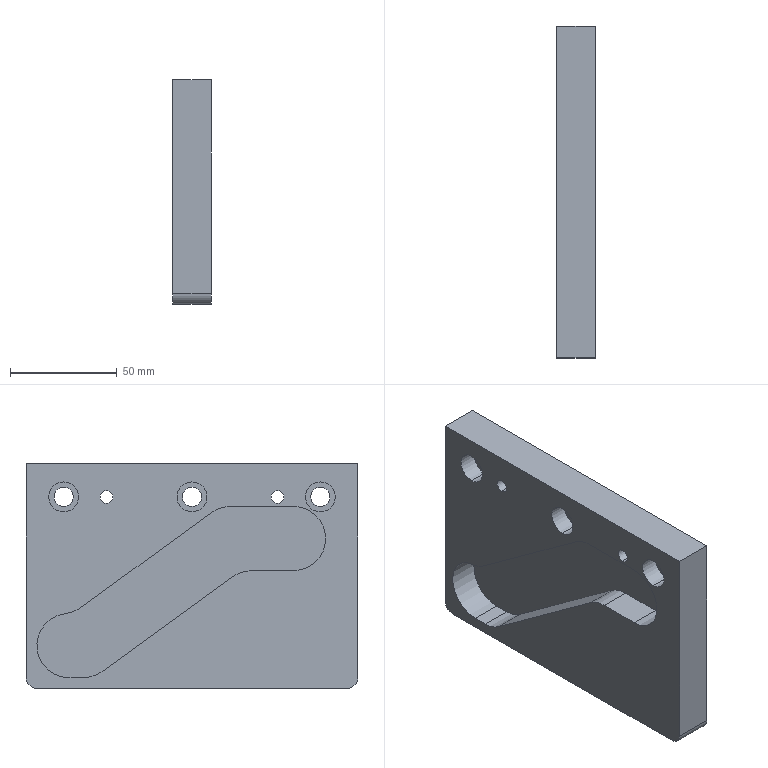Part | STEP file | LM-05-1257B | 1 solid | 39 faces | box 18 x 155 x 105 mm | volume 225163 mm3 | cylinder 24 | plane 15 | commonest cylinder face diameters 9 x6 14 x6 30 x6 6 x4 10 x2